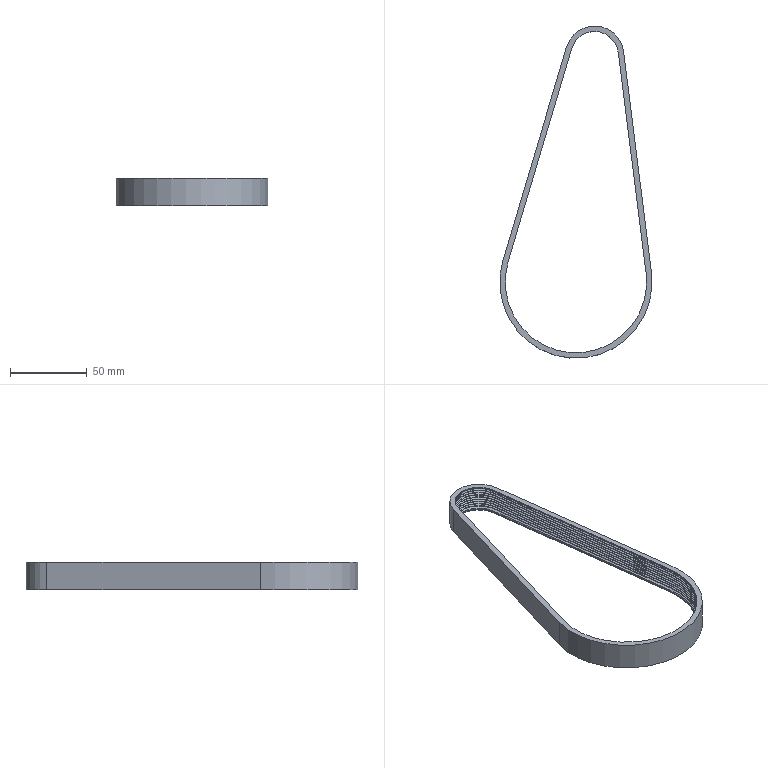Part | STEP file | DE200J601 | 1 solid | 234 faces | box 99 x 216 x 18 mm | volume 21820 mm3 | cylinder 80 | plane 62 | torus 56 | cone 36 | commonest cylinder face diameters 0.4 x52 35 x9 96 x9 1 x4 31 x2 92 x2